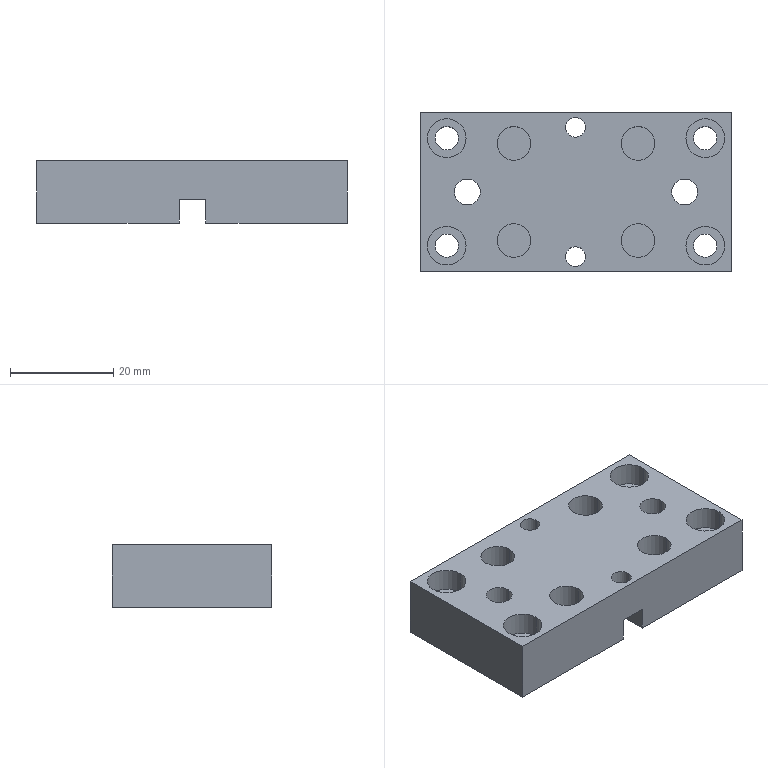Part | STEP file | Riveting base | 1 solid | 50 faces | box 60 x 30.8 x 12 mm | volume 18745 mm3 | cylinder 32 | plane 18 | commonest cylinder face diameters 4.5 x8 6.5 x8 7.5 x8 3.8 x4 5 x4